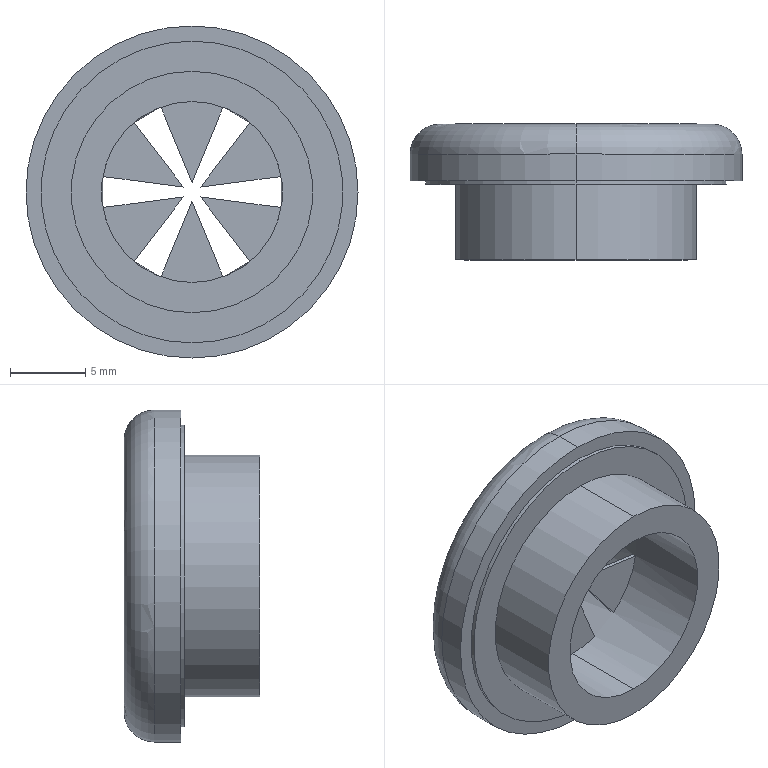Part | SolidWorks | features ICE 4, Extrusion 1, Fillet 1 | 1 solid | 38 faces | box 22 x 9 x 22 mm | volume 1452 mm3 | plane 28 | cylinder 8 | torus 2 | commonest cylinder face diameters 12 x2 16 x2 20 x2 22 x2
STEP:
#1=CARTESIAN_POINT('',(0.,7.,-11.));
#2=VERTEX_POINT('',#1);
#3=CARTESIAN_POINT('',(0.,7.,11.));
#4=VERTEX_POINT('',#3);
#5=CARTESIAN_POINT('',(0.,7.,0.));
#6=DIRECTION('',(0.,-1.,0.));
#7=DIRECTION('',(0.,0.,1.));
#8=AXIS2_PLACEMENT_3D('',#5,#6,#7);
#9=CIRCLE('',#8,11.);
#10=EDGE_CURVE('',#2,#4,#9,.T.);
#11=ORIENTED_EDGE('',*,*,#10,.F.);
#12=CARTESIAN_POINT('',(0.,9.,-9.));
#13=VERTEX_POINT('',#12);
#14=CARTESIAN_POINT('',(0.,7.,-9.));
#15=DIRECTION('',(1.,0.,0.));
#16=DIRECTION('',(0.,0.,-1.));
#17=AXIS2_PLACEMENT_3D('',#14,#15,#16);
#18=CIRCLE('',#17,2.);
#19=EDGE_CURVE('',#2,#13,#18,.T.);
#20=ORIENTED_EDGE('',*,*,#19,.T.);
#21=CARTESIAN_POINT('',(0.,9.,9.));
#22=VERTEX_POINT('',#21);
#23=CARTESIAN_POINT('',(0.,9.,0.));
#24=DIRECTION('',(0.,1.,0.));
#25=DIRECTION('',(0.,0.,1.));
#26=AXIS2_PLACEMENT_3D('',#23,#24,#25);
#27=CIRCLE('',#26,9.);
#28=EDGE_CURVE('',#22,#13,#27,.T.);
#29=ORIENTED_EDGE('',*,*,#28,.F.);
#30=CARTESIAN_POINT('',(0.,7.,9.));
#31=DIRECTION('',(-1.,0.,0.));
#32=DIRECTION('',(0.,0.,1.));
#33=AXIS2_PLACEMENT_3D('',#30,#31,#32);
#34=CIRCLE('',#33,2.);
#35=EDGE_CURVE('',#4,#22,#34,.T.);
#36=ORIENTED_EDGE('',*,*,#35,.F.);
#37=EDGE_LOOP('',(#11,#20,#29,#36));
#38=FACE_OUTER_BOUND('',#37,.T.);
#39=CARTESIAN_POINT('',(0.,7.,0.));
#40=DIRECTION('',(0.,1.,0.));
#41=DIRECTION('',(0.,0.,1.));
#42=AXIS2_PLACEMENT_3D('',#39,#40,#41);
#43=TOROIDAL_SURFACE('',#42,9.,2.);
#44=ADVANCED_FACE('',(#38),#43,.T.);
#45=CARTESIAN_POINT('',(0.,5.25,-10.));
#46=VERTEX_POINT('',#45);
#47=CARTESIAN_POINT('',(0.,5.25,10.));
#48=VERTEX_POINT('',#47);
#49=CARTESIAN_POINT('',(0.,5.25,0.));
#50=DIRECTION('',(0.,-1.,0.));
#51=DIRECTION('',(0.,0.,-1.));
#52=AXIS2_PLACEMENT_3D('',#49,#50,#51);
#53=CIRCLE('',#52,10.);
#54=EDGE_CURVE('',#46,#48,#53,.T.);
#55=ORIENTED_EDGE('',*,*,#54,.T.);
#56=CARTESIAN_POINT('',(0.,5.,10.));
#57=VERTEX_POINT('',#56);
#58=CARTESIAN_POINT('',(0.,5.25,10.));
#59=DIRECTION('',(0.,-1.,0.));
#60=VECTOR('',#59,1000.);
#61=LINE('',#58,#60);
#62=EDGE_CURVE('',#48,#57,#61,.T.);
#63=ORIENTED_EDGE('',*,*,#62,.T.);
#64=CARTESIAN_POINT('',(0.,5.,-10.));
#65=VERTEX_POINT('',#64);
#66=CARTESIAN_POINT('',(0.,5.,0.));
#67=DIRECTION('',(0.,-1.,0.));
#68=DIRECTION('',(0.,0.,-1.));
#69=AXIS2_PLACEMENT_3D('',#66,#67,#68);
#70=CIRCLE('',#69,10.);
#71=EDGE_CURVE('',#65,#57,#70,.T.);
#72=ORIENTED_EDGE('',*,*,#71,.F.);
#73=CARTESIAN_POINT('',(0.,5.25,-10.));
#74=DIRECTION('',(0.,-1.,0.));
#75=VECTOR('',#74,1000.);
#76=LINE('',#73,#75);
#77=EDGE_CURVE('',#46,#65,#76,.T.);
#78=ORIENTED_EDGE('',*,*,#77,.F.);
#79=EDGE_LOOP('',(#55,#63,#72,#78));
#80=FACE_OUTER_BOUND('',#79,.T.);
#81=CARTESIAN_POINT('',(0.,5.25,0.));
#82=DIRECTION('',(0.,-1.,0.));
#83=DIRECTION('',(0.,0.,-1.));
#84=AXIS2_PLACEMENT_3D('',#81,#82,#83);
#85=CYLINDRICAL_SURFACE('',#84,10.);
#86=ADVANCED_FACE('',(#80),#85,.T.);
#87=CARTESIAN_POINT('',(0.,5.,8.));
#88=VERTEX_POINT('',#87);
#89=CARTESIAN_POINT('',(0.,5.,-8.));
#90=VERTEX_POINT('',#89);
#91=CARTESIAN_POINT('',(0.,5.,0.));
#92=DIRECTION('',(0.,1.,0.));
#93=DIRECTION('',(0.,0.,1.));
#94=AXIS2_PLACEMENT_3D('',#91,#92,#93);
#95=CIRCLE('',#94,8.);
#96=EDGE_CURVE('',#88,#90,#95,.T.);
#97=ORIENTED_EDGE('',*,*,#96,.F.);
#98=CARTESIAN_POINT('',(0.,0.,8.));
#99=VERTEX_POINT('',#98);
#100=CARTESIAN_POINT('',(0.,5.,8.));
#101=DIRECTION('',(0.,-1.,0.));
#102=VECTOR('',#101,1000.);
#103=LINE('',#100,#102);
#104=EDGE_CURVE('',#88,#99,#103,.T.);
#105=ORIENTED_EDGE('',*,*,#104,.T.);
#106=CARTESIAN_POINT('',(0.,0.,-8.));
#107=VERTEX_POINT('',#106);
#108=CARTESIAN_POINT('',(0.,0.,0.));
#109=DIRECTION('',(0.,1.,0.));
#110=DIRECTION('',(0.,0.,1.));
#111=AXIS2_PLACEMENT_3D('',#108,#109,#110);
#112=CIRCLE('',#111,8.);
#113=EDGE_CURVE('',#99,#107,#112,.T.);
#114=ORIENTED_EDGE('',*,*,#113,.T.);
#115=CARTESIAN_POINT('',(0.,5.,-8.));
#116=DIRECTION('',(0.,-1.,0.));
#117=VECTOR('',#116,1000.);
#118=LINE('',#115,#117);
#119=EDGE_CURVE('',#90,#107,#118,.T.);
#120=ORIENTED_EDGE('',*,*,#119,.F.);
#121=EDGE_LOOP('',(#97,#105,#114,#120));
#122=FACE_OUTER_BOUND('',#121,.T.);
#123=CARTESIAN_POINT('',(0.,5.,0.));
#124=DIRECTION('',(0.,-1.,0.));
#125=DIRECTION('',(0.,0.,-1.));
#126=AXIS2_PLACEMENT_3D('',#123,#124,#125);
#127=CYLINDRICAL_SURFACE('',#126,8.);
#128=ADVANCED_FACE('',(#122),#127,.T.);
#129=CARTESIAN_POINT('',(-3.847,5.75,4.605));
#130=VERTEX_POINT('',#129);
#131=CARTESIAN_POINT('',(-5.911,5.75,1.029));
#132=VERTEX_POINT('',#131);
#133=CARTESIAN_POINT('',(0.,5.75,0.));
#134=DIRECTION('',(0.,-1.,0.));
#135=DIRECTION('',(0.,0.,1.));
#136=AXIS2_PLACEMENT_3D('',#133,#134,#135);
#137=CIRCLE('',#136,6.);
#138=EDGE_CURVE('',#130,#132,#137,.T.);
#139=ORIENTED_EDGE('',*,*,#138,.F.);
#140=CARTESIAN_POINT('',(-3.847,6.,4.605));
#141=VERTEX_POINT('',#140);
#142=CARTESIAN_POINT('',(-3.847,5.75,4.605));
#143=DIRECTION('',(0.,1.,0.));
#144=VECTOR('',#143,1000.);
#145=LINE('',#142,#144);
#146=EDGE_CURVE('',#130,#141,#145,.T.);
#147=ORIENTED_EDGE('',*,*,#146,.T.);
#148=CARTESIAN_POINT('',(-5.911,6.,1.029));
#149=VERTEX_POINT('',#148);
#150=CARTESIAN_POINT('',(0.,6.,0.));
#151=DIRECTION('',(0.,-1.,0.));
#152=DIRECTION('',(0.,0.,1.));
#153=AXIS2_PLACEMENT_3D('',#150,#151,#152);
#154=CIRCLE('',#153,6.);
#155=EDGE_CURVE('',#141,#149,#154,.T.);
#156=ORIENTED_EDGE('',*,*,#155,.T.);
#157=CARTESIAN_POINT('',(-5.911,5.75,1.029));
#158=DIRECTION('',(0.,1.,0.));
#159=VECTOR('',#158,1000.);
#160=LINE('',#157,#159);
#161=EDGE_CURVE('',#132,#149,#160,.T.);
#162=ORIENTED_EDGE('',*,*,#161,.F.);
#163=EDGE_LOOP('',(#139,#147,#156,#162));
#164=FACE_BOUND('',#163,.T.);
#165=CARTESIAN_POINT('',(-5.911,5.75,-1.029));
#166=VERTEX_POINT('',#165);
#167=CARTESIAN_POINT('',(-3.847,5.75,-4.605));
#168=VERTEX_POINT('',#167);
#169=CARTESIAN_POINT('',(0.,5.75,0.));
#170=DIRECTION('',(0.,-1.,0.));
#171=DIRECTION('',(0.,0.,1.));
#172=AXIS2_PLACEMENT_3D('',#169,#170,#171);
#173=CIRCLE('',#172,6.);
#174=EDGE_CURVE('',#166,#168,#173,.T.);
#175=ORIENTED_EDGE('',*,*,#174,.F.);
#176=CARTESIAN_POINT('',(-5.911,6.,-1.029));
#177=VERTEX_POINT('',#176);
#178=CARTESIAN_POINT('',(-5.911,5.75,-1.029));
#179=DIRECTION('',(0.,1.,0.));
#180=VECTOR('',#179,1000.);
#181=LINE('',#178,#180);
#182=EDGE_CURVE('',#166,#177,#181,.T.);
#183=ORIENTED_EDGE('',*,*,#182,.T.);
#184=CARTESIAN_POINT('',(-3.847,6.,-4.605));
#185=VERTEX_POINT('',#184);
#186=CARTESIAN_POINT('',(0.,6.,0.));
#187=DIRECTION('',(0.,-1.,0.));
#188=DIRECTION('',(0.,0.,1.));
#189=AXIS2_PLACEMENT_3D('',#186,#187,#188);
#190=CIRCLE('',#189,6.);
#191=EDGE_CURVE('',#177,#185,#190,.T.);
#192=ORIENTED_EDGE('',*,*,#191,.T.);
#193=CARTESIAN_POINT('',(-3.847,5.75,-4.605));
#194=DIRECTION('',(0.,1.,0.));
#195=VECTOR('',#194,1000.);
#196=LINE('',#193,#195);
#197=EDGE_CURVE('',#168,#185,#196,.T.);
#198=ORIENTED_EDGE('',*,*,#197,.F.);
#199=EDGE_LOOP('',(#175,#183,#192,#198));
#200=FACE_BOUND('',#199,.T.);
#201=CARTESIAN_POINT('',(0.,0.,6.));
#202=VERTEX_POINT('',#201);
#203=CARTESIAN_POINT('',(0.,0.,-6.));
#204=VERTEX_POINT('',#203);
#205=CARTESIAN_POINT('',(0.,0.,0.));
#206=DIRECTION('',(0.,-1.,0.));
#207=DIRECTION('',(0.,0.,1.));
#208=AXIS2_PLACEMENT_3D('',#205,#206,#207);
#209=CIRCLE('',#208,6.);
#210=EDGE_CURVE('',#202,#204,#209,.T.);
#211=ORIENTED_EDGE('',*,*,#210,.T.);
#212=CARTESIAN_POINT('',(0.,5.75,-6.));
#213=VERTEX_POINT('',#212);
#214=CARTESIAN_POINT('',(0.,-0.001,-6.));
#215=DIRECTION('',(0.,1.,0.));
#216=VECTOR('',#215,1000.);
#217=LINE('',#214,#216);
#218=EDGE_CURVE('',#204,#213,#217,.T.);
#219=ORIENTED_EDGE('',*,*,#218,.T.);
#220=CARTESIAN_POINT('',(-2.064,5.75,-5.634));
#221=VERTEX_POINT('',#220);
#222=CARTESIAN_POINT('',(0.,5.75,0.));
#223=DIRECTION('',(0.,-1.,0.));
#224=DIRECTION('',(0.,0.,1.));
#225=AXIS2_PLACEMENT_3D('',#222,#223,#224);
#226=CIRCLE('',#225,6.);
#227=EDGE_CURVE('',#221,#213,#226,.T.);
#228=ORIENTED_EDGE('',*,*,#227,.F.);
#229=CARTESIAN_POINT('',(-2.064,6.,-5.634));
#230=VERTEX_POINT('',#229);
#231=CARTESIAN_POINT('',(-2.064,5.75,-5.634));
#232=DIRECTION('',(0.,1.,0.));
#233=VECTOR('',#232,1000.);
#234=LINE('',#231,#233);
#235=EDGE_CURVE('',#221,#230,#234,.T.);
#236=ORIENTED_EDGE('',*,*,#235,.T.);
#237=CARTESIAN_POINT('',(0.,6.,-6.));
#238=VERTEX_POINT('',#237);
#239=CARTESIAN_POINT('',(0.,6.,0.));
#240=DIRECTION('',(0.,-1.,0.));
#241=DIRECTION('',(0.,0.,1.));
#242=AXIS2_PLACEMENT_3D('',#239,#240,#241);
#243=CIRCLE('',#242,6.);
#244=EDGE_CURVE('',#230,#238,#243,.T.);
#245=ORIENTED_EDGE('',*,*,#244,.T.);
#246=CARTESIAN_POINT('',(0.,9.,-6.));
#247=VERTEX_POINT('',#246);
#248=CARTESIAN_POINT('',(0.,-0.001,-6.));
#249=DIRECTION('',(0.,1.,0.));
#250=VECTOR('',#249,1000.);
#251=LINE('',#248,#250);
#252=EDGE_CURVE('',#238,#247,#251,.T.);
#253=ORIENTED_EDGE('',*,*,#252,.T.);
#254=CARTESIAN_POINT('',(0.,9.,6.));
#255=VERTEX_POINT('',#254);
#256=CARTESIAN_POINT('',(0.,9.,0.));
#257=DIRECTION('',(0.,1.,0.));
#258=DIRECTION('',(0.,0.,1.));
#259=AXIS2_PLACEMENT_3D('',#256,#257,#258);
#260=CIRCLE('',#259,6.);
#261=EDGE_CURVE('',#247,#255,#260,.T.);
#262=ORIENTED_EDGE('',*,*,#261,.T.);
#263=CARTESIAN_POINT('',(0.,6.,6.));
#264=VERTEX_POINT('',#263);
#265=CARTESIAN_POINT('',(0.,-0.001,6.));
#266=DIRECTION('',(0.,1.,0.));
#267=VECTOR('',#266,1000.);
#268=LINE('',#265,#267);
#269=EDGE_CURVE('',#264,#255,#268,.T.);
#270=ORIENTED_EDGE('',*,*,#269,.F.);
#271=CARTESIAN_POINT('',(-2.064,6.,5.634));
#272=VERTEX_POINT('',#271);
#273=CARTESIAN_POINT('',(0.,6.,0.));
#274=DIRECTION('',(0.,-1.,0.));
#275=DIRECTION('',(0.,0.,1.));
#276=AXIS2_PLACEMENT_3D('',#273,#274,#275);
#277=CIRCLE('',#276,6.);
#278=EDGE_CURVE('',#264,#272,#277,.T.);
#279=ORIENTED_EDGE('',*,*,#278,.T.);
#280=CARTESIAN_POINT('',(-2.064,5.75,5.634));
#281=VERTEX_POINT('',#280);
#282=CARTESIAN_POINT('',(-2.064,5.75,5.634));
#283=DIRECTION('',(0.,1.,0.));
#284=VECTOR('',#283,1000.);
#285=LINE('',#282,#284);
#286=EDGE_CURVE('',#281,#272,#285,.T.);
#287=ORIENTED_EDGE('',*,*,#286,.F.);
#288=CARTESIAN_POINT('',(0.,5.75,6.));
#289=VERTEX_POINT('',#288);
#290=CARTESIAN_POINT('',(0.,5.75,0.));
#291=DIRECTION('',(0.,-1.,0.));
#292=DIRECTION('',(0.,0.,1.));
#293=AXIS2_PLACEMENT_3D('',#290,#291,#292);
#294=CIRCLE('',#293,6.);
#295=EDGE_CURVE('',#289,#281,#294,.T.);
#296=ORIENTED_EDGE('',*,*,#295,.F.);
#297=CARTESIAN_POINT('',(0.,-0.001,6.));
#298=DIRECTION('',(0.,1.,0.));
#299=VECTOR('',#298,1000.);
#300=LINE('',#297,#299);
#301=EDGE_CURVE('',#202,#289,#300,.T.);
#302=ORIENTED_EDGE('',*,*,#301,.F.);
#303=EDGE_LOOP('',(#211,#219,#228,#236,#245,#253,#262,#270,#279,#287,#296,#302));
#304=FACE_OUTER_BOUND('',#303,.T.);
#305=CARTESIAN_POINT('',(0.,-0.001,0.));
#306=DIRECTION('',(0.,1.,0.));
#307=DIRECTION('',(0.,0.,1.));
#308=AXIS2_PLACEMENT_3D('',#305,#306,#307);
#309=CYLINDRICAL_SURFACE('',#308,6.);
#310=ADVANCED_FACE('',(#164,#200,#304),#309,.F.);
#311=ORIENTED_EDGE('',*,*,#10,.T.);
#312=CARTESIAN_POINT('',(0.,5.25,11.));
#313=VERTEX_POINT('',#312);
#314=CARTESIAN_POINT('',(0.,9.,11.));
#315=DIRECTION('',(0.,-1.,0.));
#316=VECTOR('',#315,1000.);
#317=LINE('',#314,#316);
#318=EDGE_CURVE('',#4,#313,#317,.T.);
#319=ORIENTED_EDGE('',*,*,#318,.T.);
#320=CARTESIAN_POINT('',(0.,5.25,-11.));
#321=VERTEX_POINT('',#320);
#322=CARTESIAN_POINT('',(0.,5.25,0.));
#323=DIRECTION('',(0.,-1.,0.));
#324=DIRECTION('',(0.,0.,-1.));
#325=AXIS2_PLACEMENT_3D('',#322,#323,#324);
#326=CIRCLE('',#325,11.);
#327=EDGE_CURVE('',#321,#313,#326,.T.);
#328=ORIENTED_EDGE('',*,*,#327,.F.);
#329=CARTESIAN_POINT('',(0.,9.,-11.));
#330=DIRECTION('',(0.,-1.,0.));
#331=VECTOR('',#330,1000.);
#332=LINE('',#329,#331);
#333=EDGE_CURVE('',#2,#321,#332,.T.);
#334=ORIENTED_EDGE('',*,*,#333,.F.);
#335=EDGE_LOOP('',(#311,#319,#328,#334));
#336=FACE_OUTER_BOUND('',#335,.T.);
#337=CARTESIAN_POINT('',(0.,9.,0.));
#338=DIRECTION('',(0.,-1.,0.));
#339=DIRECTION('',(0.,0.,-1.));
#340=AXIS2_PLACEMENT_3D('',#337,#338,#339);
#341=CYLINDRICAL_SURFACE('',#340,11.);
#342=ADVANCED_FACE('',(#336),#341,.T.);
#343=ORIENTED_EDGE('',*,*,#318,.F.);
#344=CARTESIAN_POINT('',(0.,7.,0.));
#345=DIRECTION('',(0.,-1.,0.));
#346=DIRECTION('',(0.,0.,1.));
#347=AXIS2_PLACEMENT_3D('',#344,#345,#346);
#348=CIRCLE('',#347,11.);
#349=EDGE_CURVE('',#4,#2,#348,.T.);
#350=ORIENTED_EDGE('',*,*,#349,.T.);
#351=ORIENTED_EDGE('',*,*,#333,.T.);
#352=CARTESIAN_POINT('',(0.,5.25,0.));
#353=DIRECTION('',(0.,-1.,0.));
#354=DIRECTION('',(0.,0.,-1.));
#355=AXIS2_PLACEMENT_3D('',#352,#353,#354);
#356=CIRCLE('',#355,11.);
#357=EDGE_CURVE('',#313,#321,#356,.T.);
#358=ORIENTED_EDGE('',*,*,#357,.F.);
#359=EDGE_LOOP('',(#343,#350,#351,#358));
#360=FACE_OUTER_BOUND('',#359,.T.);
#361=CARTESIAN_POINT('',(0.,9.,0.));
#362=DIRECTION('',(0.,-1.,0.));
#363=DIRECTION('',(0.,0.,-1.));
#364=AXIS2_PLACEMENT_3D('',#361,#362,#363);
#365=CYLINDRICAL_SURFACE('',#364,11.);
#366=ADVANCED_FACE('',(#360),#365,.T.);
#367=CARTESIAN_POINT('',(0.,5.,0.));
#368=DIRECTION('',(0.,1.,0.));
#369=DIRECTION('',(0.,0.,1.));
#370=AXIS2_PLACEMENT_3D('',#367,#368,#369);
#371=CIRCLE('',#370,8.);
#372=EDGE_CURVE('',#90,#88,#371,.T.);
#373=ORIENTED_EDGE('',*,*,#372,.T.);
#374=ORIENTED_EDGE('',*,*,#96,.T.);
#375=EDGE_LOOP('',(#373,#374));
#376=FACE_BOUND('',#375,.T.);
#377=ORIENTED_EDGE('',*,*,#71,.T.);
#378=CARTESIAN_POINT('',(0.,5.,0.));
#379=DIRECTION('',(0.,-1.,0.));
#380=DIRECTION('',(0.,0.,-1.));
#381=AXIS2_PLACEMENT_3D('',#378,#379,#380);
#382=CIRCLE('',#381,10.);
#383=EDGE_CURVE('',#57,#65,#382,.T.);
#384=ORIENTED_EDGE('',*,*,#383,.T.);
#385=EDGE_LOOP('',(#377,#384));
#386=FACE_OUTER_BOUND('',#385,.T.);
#387=CARTESIAN_POINT('',(0.,5.,0.));
#388=DIRECTION('',(0.,1.,0.));
#389=DIRECTION('',(0.,0.,1.));
#390=AXIS2_PLACEMENT_3D('',#387,#388,#389);
#391=PLANE('',#390);
#392=ADVANCED_FACE('',(#376,#386),#391,.F.);
#393=ORIENTED_EDGE('',*,*,#218,.F.);
#394=CARTESIAN_POINT('',(0.,0.,0.));
#395=DIRECTION('',(0.,-1.,0.));
#396=DIRECTION('',(0.,0.,1.));
#397=AXIS2_PLACEMENT_3D('',#394,#395,#396);
#398=CIRCLE('',#397,6.);
#399=EDGE_CURVE('',#204,#202,#398,.T.);
#400=ORIENTED_EDGE('',*,*,#399,.T.);
#401=ORIENTED_EDGE('',*,*,#301,.T.);
#402=CARTESIAN_POINT('',(2.064,5.75,5.634));
#403=VERTEX_POINT('',#402);
#404=CARTESIAN_POINT('',(0.,5.75,0.));
#405=DIRECTION('',(0.,-1.,0.));
#406=DIRECTION('',(0.,0.,1.));
#407=AXIS2_PLACEMENT_3D('',#404,#405,#406);
#408=CIRCLE('',#407,6.);
#409=EDGE_CURVE('',#403,#289,#408,.T.);
#410=ORIENTED_EDGE('',*,*,#409,.F.);
#411=CARTESIAN_POINT('',(2.064,6.,5.634));
#412=VERTEX_POINT('',#411);
#413=CARTESIAN_POINT('',(2.064,5.75,5.634));
#414=DIRECTION('',(0.,1.,0.));
#415=VECTOR('',#414,1000.);
#416=LINE('',#413,#415);
#417=EDGE_CURVE('',#403,#412,#416,.T.);
#418=ORIENTED_EDGE('',*,*,#417,.T.);
#419=CARTESIAN_POINT('',(0.,6.,0.));
#420=DIRECTION('',(0.,-1.,0.));
#421=DIRECTION('',(0.,0.,1.));
#422=AXIS2_PLACEMENT_3D('',#419,#420,#421);
#423=CIRCLE('',#422,6.);
#424=EDGE_CURVE('',#412,#264,#423,.T.);
#425=ORIENTED_EDGE('',*,*,#424,.T.);
#426=ORIENTED_EDGE('',*,*,#269,.T.);
#427=CARTESIAN_POINT('',(0.,9.,0.));
#428=DIRECTION('',(0.,1.,0.));
#429=DIRECTION('',(0.,0.,1.));
#430=AXIS2_PLACEMENT_3D('',#427,#428,#429);
#431=CIRCLE('',#430,6.);
#432=EDGE_CURVE('',#255,#247,#431,.T.);
#433=ORIENTED_EDGE('',*,*,#432,.T.);
#434=ORIENTED_EDGE('',*,*,#252,.F.);
#435=CARTESIAN_POINT('',(2.064,6.,-5.634));
#436=VERTEX_POINT('',#435);
#437=CARTESIAN_POINT('',(0.,6.,0.));
#438=DIRECTION('',(0.,-1.,0.));
#439=DIRECTION('',(0.,0.,1.));
#440=AXIS2_PLACEMENT_3D('',#437,#438,#439);
#441=CIRCLE('',#440,6.);
#442=EDGE_CURVE('',#238,#436,#441,.T.);
#443=ORIENTED_EDGE('',*,*,#442,.T.);
#444=CARTESIAN_POINT('',(2.064,5.75,-5.634));
#445=VERTEX_POINT('',#444);
#446=CARTESIAN_POINT('',(2.064,5.75,-5.634));
#447=DIRECTION('',(0.,1.,0.));
#448=VECTOR('',#447,1000.);
#449=LINE('',#446,#448);
#450=EDGE_CURVE('',#445,#436,#449,.T.);
#451=ORIENTED_EDGE('',*,*,#450,.F.);
#452=CARTESIAN_POINT('',(0.,5.75,0.));
#453=DIRECTION('',(0.,-1.,0.));
#454=DIRECTION('',(0.,0.,1.));
#455=AXIS2_PLACEMENT_3D('',#452,#453,#454);
#456=CIRCLE('',#455,6.);
#457=EDGE_CURVE('',#213,#445,#456,.T.);
#458=ORIENTED_EDGE('',*,*,#457,.F.);
#459=EDGE_LOOP('',(#393,#400,#401,#410,#418,#425,#426,#433,#434,#443,#451,#458));
#460=FACE_OUTER_BOUND('',#459,.T.);
#461=CARTESIAN_POINT('',(3.847,5.75,-4.605));
#462=VERTEX_POINT('',#461);
#463=CARTESIAN_POINT('',(5.911,5.75,-1.029));
#464=VERTEX_POINT('',#463);
#465=CARTESIAN_POINT('',(0.,5.75,0.));
#466=DIRECTION('',(0.,-1.,0.));
#467=DIRECTION('',(0.,0.,1.));
#468=AXIS2_PLACEMENT_3D('',#465,#466,#467);
#469=CIRCLE('',#468,6.);
#470=EDGE_CURVE('',#462,#464,#469,.T.);
#471=ORIENTED_EDGE('',*,*,#470,.F.);
#472=CARTESIAN_POINT('',(3.847,6.,-4.605));
#473=VERTEX_POINT('',#472);
#474=CARTESIAN_POINT('',(3.847,5.75,-4.605));
#475=DIRECTION('',(0.,1.,0.));
#476=VECTOR('',#475,1000.);
#477=LINE('',#474,#476);
#478=EDGE_CURVE('',#462,#473,#477,.T.);
#479=ORIENTED_EDGE('',*,*,#478,.T.);
#480=CARTESIAN_POINT('',(5.911,6.,-1.029));
#481=VERTEX_POINT('',#480);
#482=CARTESIAN_POINT('',(0.,6.,0.));
#483=DIRECTION('',(0.,-1.,0.));
#484=DIRECTION('',(0.,0.,1.));
#485=AXIS2_PLACEMENT_3D('',#482,#483,#484);
#486=CIRCLE('',#485,6.);
#487=EDGE_CURVE('',#473,#481,#486,.T.);
#488=ORIENTED_EDGE('',*,*,#487,.T.);
#489=CARTESIAN_POINT('',(5.911,5.75,-1.029));
#490=DIRECTION('',(0.,1.,0.));
#491=VECTOR('',#490,1000.);
#492=LINE('',#489,#491);
#493=EDGE_CURVE('',#464,#481,#492,.T.);
#494=ORIENTED_EDGE('',*,*,#493,.F.);
#495=EDGE_LOOP('',(#471,#479,#488,#494));
#496=FACE_BOUND('',#495,.T.);
#497=CARTESIAN_POINT('',(5.911,5.75,1.029));
#498=VERTEX_POINT('',#497);
#499=CARTESIAN_POINT('',(3.847,5.75,4.605));
#500=VERTEX_POINT('',#499);
#501=CARTESIAN_POINT('',(0.,5.75,0.));
#502=DIRECTION('',(0.,-1.,0.));
#503=DIRECTION('',(0.,0.,1.));
#504=AXIS2_PLACEMENT_3D('',#501,#502,#503);
#505=CIRCLE('',#504,6.);
#506=EDGE_CURVE('',#498,#500,#505,.T.);
#507=ORIENTED_EDGE('',*,*,#506,.F.);
#508=CARTESIAN_POINT('',(5.911,6.,1.029));
#509=VERTEX_POINT('',#508);
#510=CARTESIAN_POINT('',(5.911,5.75,1.029));
#511=DIRECTION('',(0.,1.,0.));
#512=VECTOR('',#511,1000.);
#513=LINE('',#510,#512);
#514=EDGE_CURVE('',#498,#509,#513,.T.);
#515=ORIENTED_EDGE('',*,*,#514,.T.);
#516=CARTESIAN_POINT('',(3.847,6.,4.605));
#517=VERTEX_POINT('',#516);
#518=CARTESIAN_POINT('',(0.,6.,0.));
#519=DIRECTION('',(0.,-1.,0.));
#520=DIRECTION('',(0.,0.,1.));
#521=AXIS2_PLACEMENT_3D('',#518,#519,#520);
#522=CIRCLE('',#521,6.);
#523=EDGE_CURVE('',#509,#517,#522,.T.);
#524=ORIENTED_EDGE('',*,*,#523,.T.);
#525=CARTESIAN_POINT('',(3.847,5.75,4.605));
#526=DIRECTION('',(0.,1.,0.));
#527=VECTOR('',#526,1000.);
#528=LINE('',#525,#527);
#529=EDGE_CURVE('',#500,#517,#528,.T.);
#530=ORIENTED_EDGE('',*,*,#529,.F.);
#531=EDGE_LOOP('',(#507,#515,#524,#530));
#532=FACE_BOUND('',#531,.T.);
#533=CARTESIAN_POINT('',(0.,-0.001,0.));
#534=DIRECTION('',(0.,1.,0.));
#535=DIRECTION('',(0.,0.,1.));
#536=AXIS2_PLACEMENT_3D('',#533,#534,#535);
#537=CYLINDRICAL_SURFACE('',#536,6.);
#538=ADVANCED_FACE('',(#460,#496,#532),#537,.F.);
#539=ORIENTED_EDGE('',*,*,#104,.F.);
#540=ORIENTED_EDGE('',*,*,#372,.F.);
#541=ORIENTED_EDGE('',*,*,#119,.T.);
#542=CARTESIAN_POINT('',(0.,0.,0.));
#543=DIRECTION('',(0.,1.,0.));
#544=DIRECTION('',(0.,0.,1.));
#545=AXIS2_PLACEMENT_3D('',#542,#543,#544);
#546=CIRCLE('',#545,8.);
#547=EDGE_CURVE('',#107,#99,#546,.T.);
#548=ORIENTED_EDGE('',*,*,#547,.T.);
#549=EDGE_LOOP('',(#539,#540,#541,#548));
#550=FACE_OUTER_BOUND('',#549,.T.);
#551=CARTESIAN_POINT('',(0.,5.,0.));
#552=DIRECTION('',(0.,-1.,0.));
#553=DIRECTION('',(0.,0.,-1.));
#554=AXIS2_PLACEMENT_3D('',#551,#552,#553);
#555=CYLINDRICAL_SURFACE('',#554,8.);
#556=ADVANCED_FACE('',(#550),#555,.T.);
#557=ORIENTED_EDGE('',*,*,#210,.F.);
#558=ORIENTED_EDGE('',*,*,#399,.F.);
#559=EDGE_LOOP('',(#557,#558));
#560=FACE_BOUND('',#559,.T.);
#561=ORIENTED_EDGE('',*,*,#547,.F.);
#562=ORIENTED_EDGE('',*,*,#113,.F.);
#563=EDGE_LOOP('',(#561,#562));
#564=FACE_OUTER_BOUND('',#563,.T.);
#565=CARTESIAN_POINT('',(0.,0.,0.));
#566=DIRECTION('',(0.,1.,0.));
#567=DIRECTION('',(0.,0.,1.));
#568=AXIS2_PLACEMENT_3D('',#565,#566,#567);
#569=PLANE('',#568);
#570=ADVANCED_FACE('',(#560,#564),#569,.F.);
#571=ORIENTED_EDGE('',*,*,#28,.T.);
#572=CARTESIAN_POINT('',(0.,9.,0.));
#573=DIRECTION('',(0.,1.,0.));
#574=DIRECTION('',(0.,0.,1.));
#575=AXIS2_PLACEMENT_3D('',#572,#573,#574);
#576=CIRCLE('',#575,9.);
#577=EDGE_CURVE('',#13,#22,#576,.T.);
#578=ORIENTED_EDGE('',*,*,#577,.T.);
#579=EDGE_LOOP('',(#571,#578));
#580=FACE_OUTER_BOUND('',#579,.T.);
#581=ORIENTED_EDGE('',*,*,#432,.F.);
#582=ORIENTED_EDGE('',*,*,#261,.F.);
#583=EDGE_LOOP('',(#581,#582));
#584=FACE_BOUND('',#583,.T.);
#585=CARTESIAN_POINT('',(0.,9.,0.));
#586=DIRECTION('',(0.,1.,0.));
#587=DIRECTION('',(0.,0.,1.));
#588=AXIS2_PLACEMENT_3D('',#585,#586,#587);
#589=PLANE('',#588);
#590=ADVANCED_FACE('',(#580,#584),#589,.T.);
#591=CARTESIAN_POINT('',(0.,6.,0.65));
#592=VERTEX_POINT('',#591);
#593=CARTESIAN_POINT('',(0.,6.,0.65));
#594=DIRECTION('',(0.3827,0.,0.9239));
#595=VECTOR('',#594,1000.);
#596=LINE('',#593,#595);
#597=EDGE_CURVE('',#592,#412,#596,.T.);
#598=ORIENTED_EDGE('',*,*,#597,.T.);
#599=ORIENTED_EDGE('',*,*,#417,.F.);
#600=CARTESIAN_POINT('',(0.,5.75,0.65));
#601=VERTEX_POINT('',#600);
#602=CARTESIAN_POINT('',(0.,5.75,0.65));
#603=DIRECTION('',(0.3827,0.,0.9239));
#604=VECTOR('',#603,1000.);
#605=LINE('',#602,#604);
#606=EDGE_CURVE('',#601,#403,#605,.T.);
#607=ORIENTED_EDGE('',*,*,#606,.F.);
#608=CARTESIAN_POINT('',(0.,5.75,0.65));
#609=DIRECTION('',(0.,1.,0.));
#610=VECTOR('',#609,1000.);
#611=LINE('',#608,#610);
#612=EDGE_CURVE('',#601,#592,#611,.T.);
#613=ORIENTED_EDGE('',*,*,#612,.T.);
#614=EDGE_LOOP('',(#598,#599,#607,#613));
#615=FACE_OUTER_BOUND('',#614,.T.);
#616=CARTESIAN_POINT('',(0.,5.75,0.65));
#617=DIRECTION('',(-0.9239,0.,0.3827));
#618=DIRECTION('',(0.3827,0.,0.9239));
#619=AXIS2_PLACEMENT_3D('',#616,#617,#618);
#620=PLANE('',#619);
#621=ADVANCED_FACE('',(#615),#620,.F.);
#622=CARTESIAN_POINT('',(0.,6.,0.65));
#623=DIRECTION('',(0.3827,0.,-0.9239));
#624=VECTOR('',#623,1000.);
#625=LINE('',#622,#624);
#626=EDGE_CURVE('',#272,#592,#625,.T.);
#627=ORIENTED_EDGE('',*,*,#626,.T.);
#628=ORIENTED_EDGE('',*,*,#612,.F.);
#629=CARTESIAN_POINT('',(0.,5.75,0.65));
#630=DIRECTION('',(0.3827,0.,-0.9239));
#631=VECTOR('',#630,1000.);
#632=LINE('',#629,#631);
#633=EDGE_CURVE('',#281,#601,#632,.T.);
#634=ORIENTED_EDGE('',*,*,#633,.F.);
#635=ORIENTED_EDGE('',*,*,#286,.T.);
#636=EDGE_LOOP('',(#627,#628,#634,#635));
#637=FACE_OUTER_BOUND('',#636,.T.);
#638=CARTESIAN_POINT('',(0.,5.75,0.65));
#639=DIRECTION('',(0.9239,0.,0.3827));
#640=DIRECTION('',(0.3827,0.,-0.9239));
#641=AXIS2_PLACEMENT_3D('',#638,#639,#640);
#642=PLANE('',#641);
#643=ADVANCED_FACE('',(#637),#642,.F.);
#644=ORIENTED_EDGE('',*,*,#606,.T.);
#645=ORIENTED_EDGE('',*,*,#409,.T.);
#646=ORIENTED_EDGE('',*,*,#295,.T.);
#647=ORIENTED_EDGE('',*,*,#633,.T.);
#648=EDGE_LOOP('',(#644,#645,#646,#647));
#649=FACE_OUTER_BOUND('',#648,.T.);
#650=CARTESIAN_POINT('',(0.,5.75,0.));
#651=DIRECTION('',(0.,1.,0.));
#652=DIRECTION('',(0.,0.,1.));
#653=AXIS2_PLACEMENT_3D('',#650,#651,#652);
#654=PLANE('',#653);
#655=ADVANCED_FACE('',(#649),#654,.F.);
#656=ORIENTED_EDGE('',*,*,#597,.F.);
#657=ORIENTED_EDGE('',*,*,#626,.F.);
#658=ORIENTED_EDGE('',*,*,#278,.F.);
#659=ORIENTED_EDGE('',*,*,#424,.F.);
#660=EDGE_LOOP('',(#656,#657,#658,#659));
#661=FACE_OUTER_BOUND('',#660,.T.);
#662=CARTESIAN_POINT('',(0.,6.,0.));
#663=DIRECTION('',(0.,1.,0.));
#664=DIRECTION('',(0.,0.,1.));
#665=AXIS2_PLACEMENT_3D('',#662,#663,#664);
#666=PLANE('',#665);
#667=ADVANCED_FACE('',(#661),#666,.T.);
#668=CARTESIAN_POINT('',(0.5629,6.,0.325));
#669=VERTEX_POINT('',#668);
#670=CARTESIAN_POINT('',(0.5629,6.,0.325));
#671=DIRECTION('',(0.9914,0.,0.1305));
#672=VECTOR('',#671,1000.);
#673=LINE('',#670,#672);
#674=EDGE_CURVE('',#669,#509,#673,.T.);
#675=ORIENTED_EDGE('',*,*,#674,.T.);
#676=ORIENTED_EDGE('',*,*,#514,.F.);
#677=CARTESIAN_POINT('',(0.5629,5.75,0.325));
#678=VERTEX_POINT('',#677);
#679=CARTESIAN_POINT('',(0.5629,5.75,0.325));
#680=DIRECTION('',(0.9914,0.,0.1305));
#681=VECTOR('',#680,1000.);
#682=LINE('',#679,#681);
#683=EDGE_CURVE('',#678,#498,#682,.T.);
#684=ORIENTED_EDGE('',*,*,#683,.F.);
#685=CARTESIAN_POINT('',(0.5629,5.75,0.325));
#686=DIRECTION('',(0.,1.,0.));
#687=VECTOR('',#686,1000.);
#688=LINE('',#685,#687);
#689=EDGE_CURVE('',#678,#669,#688,.T.);
#690=ORIENTED_EDGE('',*,*,#689,.T.);
#691=EDGE_LOOP('',(#675,#676,#684,#690));
#692=FACE_OUTER_BOUND('',#691,.T.);
#693=CARTESIAN_POINT('',(0.5629,5.75,0.325));
#694=DIRECTION('',(-0.1305,0.,0.9914));
#695=DIRECTION('',(0.9914,0.,0.1305));
#696=AXIS2_PLACEMENT_3D('',#693,#694,#695);
#697=PLANE('',#696);
#698=ADVANCED_FACE('',(#692),#697,.F.);
#699=CARTESIAN_POINT('',(0.5629,6.,0.325));
#700=DIRECTION('',(-0.6088,0.,-0.7934));
#701=VECTOR('',#700,1000.);
#702=LINE('',#699,#701);
#703=EDGE_CURVE('',#517,#669,#702,.T.);
#704=ORIENTED_EDGE('',*,*,#703,.T.);
#705=ORIENTED_EDGE('',*,*,#689,.F.);
#706=CARTESIAN_POINT('',(0.5629,5.75,0.325));
#707=DIRECTION('',(-0.6088,0.,-0.7934));
#708=VECTOR('',#707,1000.);
#709=LINE('',#706,#708);
#710=EDGE_CURVE('',#500,#678,#709,.T.);
#711=ORIENTED_EDGE('',*,*,#710,.F.);
#712=ORIENTED_EDGE('',*,*,#529,.T.);
#713=EDGE_LOOP('',(#704,#705,#711,#712));
#714=FACE_OUTER_BOUND('',#713,.T.);
#715=CARTESIAN_POINT('',(0.5629,5.75,0.325));
#716=DIRECTION('',(0.7934,0.,-0.6088));
#717=DIRECTION('',(-0.6088,0.,-0.7934));
#718=AXIS2_PLACEMENT_3D('',#715,#716,#717);
#719=PLANE('',#718);
#720=ADVANCED_FACE('',(#714),#719,.F.);
#721=ORIENTED_EDGE('',*,*,#683,.T.);
#722=ORIENTED_EDGE('',*,*,#506,.T.);
#723=ORIENTED_EDGE('',*,*,#710,.T.);
#724=EDGE_LOOP('',(#721,#722,#723));
#725=FACE_OUTER_BOUND('',#724,.T.);
#726=CARTESIAN_POINT('',(0.,5.75,0.));
#727=DIRECTION('',(0.,1.,0.));
#728=DIRECTION('',(0.,0.,1.));
#729=AXIS2_PLACEMENT_3D('',#726,#727,#728);
#730=PLANE('',#729);
#731=ADVANCED_FACE('',(#725),#730,.F.);
#732=ORIENTED_EDGE('',*,*,#674,.F.);
#733=ORIENTED_EDGE('',*,*,#703,.F.);
#734=ORIENTED_EDGE('',*,*,#523,.F.);
#735=EDGE_LOOP('',(#732,#733,#734));
#736=FACE_OUTER_BOUND('',#735,.T.);
#737=CARTESIAN_POINT('',(0.,6.,0.));
#738=DIRECTION('',(0.,1.,0.));
#739=DIRECTION('',(0.,0.,1.));
#740=AXIS2_PLACEMENT_3D('',#737,#738,#739);
#741=PLANE('',#740);
#742=ADVANCED_FACE('',(#736),#741,.T.);
#743=CARTESIAN_POINT('',(0.5629,6.,-0.325));
#744=VERTEX_POINT('',#743);
#745=CARTESIAN_POINT('',(0.5629,6.,-0.325));
#746=DIRECTION('',(0.6088,0.,-0.7934));
#747=VECTOR('',#746,1000.);
#748=LINE('',#745,#747);
#749=EDGE_CURVE('',#744,#473,#748,.T.);
#750=ORIENTED_EDGE('',*,*,#749,.T.);
#751=ORIENTED_EDGE('',*,*,#478,.F.);
#752=CARTESIAN_POINT('',(0.5629,5.75,-0.325));
#753=VERTEX_POINT('',#752);
#754=CARTESIAN_POINT('',(0.5629,5.75,-0.325));
#755=DIRECTION('',(0.6088,0.,-0.7934));
#756=VECTOR('',#755,1000.);
#757=LINE('',#754,#756);
#758=EDGE_CURVE('',#753,#462,#757,.T.);
#759=ORIENTED_EDGE('',*,*,#758,.F.);
#760=CARTESIAN_POINT('',(0.5629,5.75,-0.325));
#761=DIRECTION('',(0.,1.,0.));
#762=VECTOR('',#761,1000.);
#763=LINE('',#760,#762);
#764=EDGE_CURVE('',#753,#744,#763,.T.);
#765=ORIENTED_EDGE('',*,*,#764,.T.);
#766=EDGE_LOOP('',(#750,#751,#759,#765));
#767=FACE_OUTER_BOUND('',#766,.T.);
#768=CARTESIAN_POINT('',(0.5629,5.75,-0.325));
#769=DIRECTION('',(0.7934,0.,0.6088));
#770=DIRECTION('',(0.6088,0.,-0.7934));
#771=AXIS2_PLACEMENT_3D('',#768,#769,#770);
#772=PLANE('',#771);
#773=ADVANCED_FACE('',(#767),#772,.F.);
#774=CARTESIAN_POINT('',(0.5629,6.,-0.325));
#775=DIRECTION('',(-0.9914,0.,0.1305));
#776=VECTOR('',#775,1000.);
#777=LINE('',#774,#776);
#778=EDGE_CURVE('',#481,#744,#777,.T.);
#779=ORIENTED_EDGE('',*,*,#778,.T.);
#780=ORIENTED_EDGE('',*,*,#764,.F.);
#781=CARTESIAN_POINT('',(0.5629,5.75,-0.325));
#782=DIRECTION('',(-0.9914,0.,0.1305));
#783=VECTOR('',#782,1000.);
#784=LINE('',#781,#783);
#785=EDGE_CURVE('',#464,#753,#784,.T.);
#786=ORIENTED_EDGE('',*,*,#785,.F.);
#787=ORIENTED_EDGE('',*,*,#493,.T.);
#788=EDGE_LOOP('',(#779,#780,#786,#787));
#789=FACE_OUTER_BOUND('',#788,.T.);
#790=CARTESIAN_POINT('',(0.5629,5.75,-0.325));
#791=DIRECTION('',(-0.1305,0.,-0.9914));
#792=DIRECTION('',(-0.9914,0.,0.1305));
#793=AXIS2_PLACEMENT_3D('',#790,#791,#792);
#794=PLANE('',#793);
#795=ADVANCED_FACE('',(#789),#794,.F.);
#796=ORIENTED_EDGE('',*,*,#758,.T.);
#797=ORIENTED_EDGE('',*,*,#470,.T.);
#798=ORIENTED_EDGE('',*,*,#785,.T.);
#799=EDGE_LOOP('',(#796,#797,#798));
#800=FACE_OUTER_BOUND('',#799,.T.);
#801=CARTESIAN_POINT('',(0.,5.75,0.));
#802=DIRECTION('',(0.,1.,0.));
#803=DIRECTION('',(0.,0.,1.));
#804=AXIS2_PLACEMENT_3D('',#801,#802,#803);
#805=PLANE('',#804);
#806=ADVANCED_FACE('',(#800),#805,.F.);
#807=ORIENTED_EDGE('',*,*,#749,.F.);
#808=ORIENTED_EDGE('',*,*,#778,.F.);
#809=ORIENTED_EDGE('',*,*,#487,.F.);
#810=EDGE_LOOP('',(#807,#808,#809));
#811=FACE_OUTER_BOUND('',#810,.T.);
#812=CARTESIAN_POINT('',(0.,6.,0.));
#813=DIRECTION('',(0.,1.,0.));
#814=DIRECTION('',(0.,0.,1.));
#815=AXIS2_PLACEMENT_3D('',#812,#813,#814);
#816=PLANE('',#815);
#817=ADVANCED_FACE('',(#811),#816,.T.);
#818=CARTESIAN_POINT('',(0.,6.,-0.65));
#819=VERTEX_POINT('',#818);
#820=CARTESIAN_POINT('',(0.,6.,-0.65));
#821=DIRECTION('',(-0.3827,0.,-0.9239));
#822=VECTOR('',#821,1000.);
#823=LINE('',#820,#822);
#824=EDGE_CURVE('',#819,#230,#823,.T.);
#825=ORIENTED_EDGE('',*,*,#824,.T.);
#826=ORIENTED_EDGE('',*,*,#235,.F.);
#827=CARTESIAN_POINT('',(0.,5.75,-0.65));
#828=VERTEX_POINT('',#827);
#829=CARTESIAN_POINT('',(0.,5.75,-0.65));
#830=DIRECTION('',(-0.3827,0.,-0.9239));
#831=VECTOR('',#830,1000.);
#832=LINE('',#829,#831);
#833=EDGE_CURVE('',#828,#221,#832,.T.);
#834=ORIENTED_EDGE('',*,*,#833,.F.);
#835=CARTESIAN_POINT('',(0.,5.75,-0.65));
#836=DIRECTION('',(0.,1.,0.));
#837=VECTOR('',#836,1000.);
#838=LINE('',#835,#837);
#839=EDGE_CURVE('',#828,#819,#838,.T.);
#840=ORIENTED_EDGE('',*,*,#839,.T.);
#841=EDGE_LOOP('',(#825,#826,#834,#840));
#842=FACE_OUTER_BOUND('',#841,.T.);
#843=CARTESIAN_POINT('',(0.,5.75,-0.65));
#844=DIRECTION('',(0.9239,0.,-0.3827));
#845=DIRECTION('',(-0.3827,0.,-0.9239));
#846=AXIS2_PLACEMENT_3D('',#843,#844,#845);
#847=PLANE('',#846);
#848=ADVANCED_FACE('',(#842),#847,.F.);
#849=CARTESIAN_POINT('',(0.,6.,-0.65));
#850=DIRECTION('',(-0.3827,0.,0.9239));
#851=VECTOR('',#850,1000.);
#852=LINE('',#849,#851);
#853=EDGE_CURVE('',#436,#819,#852,.T.);
#854=ORIENTED_EDGE('',*,*,#853,.T.);
#855=ORIENTED_EDGE('',*,*,#839,.F.);
#856=CARTESIAN_POINT('',(0.,5.75,-0.65));
#857=DIRECTION('',(-0.3827,0.,0.9239));
#858=VECTOR('',#857,1000.);
#859=LINE('',#856,#858);
#860=EDGE_CURVE('',#445,#828,#859,.T.);
#861=ORIENTED_EDGE('',*,*,#860,.F.);
#862=ORIENTED_EDGE('',*,*,#450,.T.);
#863=EDGE_LOOP('',(#854,#855,#861,#862));
#864=FACE_OUTER_BOUND('',#863,.T.);
#865=CARTESIAN_POINT('',(0.,5.75,-0.65));
#866=DIRECTION('',(-0.9239,0.,-0.3827));
#867=DIRECTION('',(-0.3827,0.,0.9239));
#868=AXIS2_PLACEMENT_3D('',#865,#866,#867);
#869=PLANE('',#868);
#870=ADVANCED_FACE('',(#864),#869,.F.);
#871=ORIENTED_EDGE('',*,*,#833,.T.);
#872=ORIENTED_EDGE('',*,*,#227,.T.);
#873=ORIENTED_EDGE('',*,*,#457,.T.);
#874=ORIENTED_EDGE('',*,*,#860,.T.);
#875=EDGE_LOOP('',(#871,#872,#873,#874));
#876=FACE_OUTER_BOUND('',#875,.T.);
#877=CARTESIAN_POINT('',(0.,5.75,0.));
#878=DIRECTION('',(0.,1.,0.));
#879=DIRECTION('',(0.,0.,1.));
#880=AXIS2_PLACEMENT_3D('',#877,#878,#879);
#881=PLANE('',#880);
#882=ADVANCED_FACE('',(#876),#881,.F.);
#883=ORIENTED_EDGE('',*,*,#824,.F.);
#884=ORIENTED_EDGE('',*,*,#853,.F.);
#885=ORIENTED_EDGE('',*,*,#442,.F.);
#886=ORIENTED_EDGE('',*,*,#244,.F.);
#887=EDGE_LOOP('',(#883,#884,#885,#886));
#888=FACE_OUTER_BOUND('',#887,.T.);
#889=CARTESIAN_POINT('',(0.,6.,0.));
#890=DIRECTION('',(0.,1.,0.));
#891=DIRECTION('',(0.,0.,1.));
#892=AXIS2_PLACEMENT_3D('',#889,#890,#891);
#893=PLANE('',#892);
#894=ADVANCED_FACE('',(#888),#893,.T.);
#895=CARTESIAN_POINT('',(-0.5629,6.,-0.325));
#896=VERTEX_POINT('',#895);
#897=CARTESIAN_POINT('',(-0.5629,6.,-0.325));
#898=DIRECTION('',(-0.9914,0.,-0.1305));
#899=VECTOR('',#898,1000.);
#900=LINE('',#897,#899);
#901=EDGE_CURVE('',#896,#177,#900,.T.);
#902=ORIENTED_EDGE('',*,*,#901,.T.);
#903=ORIENTED_EDGE('',*,*,#182,.F.);
#904=CARTESIAN_POINT('',(-0.5629,5.75,-0.325));
#905=VERTEX_POINT('',#904);
#906=CARTESIAN_POINT('',(-0.5629,5.75,-0.325));
#907=DIRECTION('',(-0.9914,0.,-0.1305));
#908=VECTOR('',#907,1000.);
#909=LINE('',#906,#908);
#910=EDGE_CURVE('',#905,#166,#909,.T.);
#911=ORIENTED_EDGE('',*,*,#910,.F.);
#912=CARTESIAN_POINT('',(-0.5629,5.75,-0.325));
#913=DIRECTION('',(0.,1.,0.));
#914=VECTOR('',#913,1000.);
#915=LINE('',#912,#914);
#916=EDGE_CURVE('',#905,#896,#915,.T.);
#917=ORIENTED_EDGE('',*,*,#916,.T.);
#918=EDGE_LOOP('',(#902,#903,#911,#917));
#919=FACE_OUTER_BOUND('',#918,.T.);
#920=CARTESIAN_POINT('',(-0.5629,5.75,-0.325));
#921=DIRECTION('',(0.1305,0.,-0.9914));
#922=DIRECTION('',(-0.9914,0.,-0.1305));
#923=AXIS2_PLACEMENT_3D('',#920,#921,#922);
#924=PLANE('',#923);
#925=ADVANCED_FACE('',(#919),#924,.F.);
#926=CARTESIAN_POINT('',(-0.5629,6.,-0.325));
#927=DIRECTION('',(0.6088,0.,0.7934));
#928=VECTOR('',#927,1000.);
#929=LINE('',#926,#928);
#930=EDGE_CURVE('',#185,#896,#929,.T.);
#931=ORIENTED_EDGE('',*,*,#930,.T.);
#932=ORIENTED_EDGE('',*,*,#916,.F.);
#933=CARTESIAN_POINT('',(-0.5629,5.75,-0.325));
#934=DIRECTION('',(0.6088,0.,0.7934));
#935=VECTOR('',#934,1000.);
#936=LINE('',#933,#935);
#937=EDGE_CURVE('',#168,#905,#936,.T.);
#938=ORIENTED_EDGE('',*,*,#937,.F.);
#939=ORIENTED_EDGE('',*,*,#197,.T.);
#940=EDGE_LOOP('',(#931,#932,#938,#939));
#941=FACE_OUTER_BOUND('',#940,.T.);
#942=CARTESIAN_POINT('',(-0.5629,5.75,-0.325));
#943=DIRECTION('',(-0.7934,0.,0.6088));
#944=DIRECTION('',(0.6088,0.,0.7934));
#945=AXIS2_PLACEMENT_3D('',#942,#943,#944);
#946=PLANE('',#945);
#947=ADVANCED_FACE('',(#941),#946,.F.);
#948=ORIENTED_EDGE('',*,*,#910,.T.);
#949=ORIENTED_EDGE('',*,*,#174,.T.);
#950=ORIENTED_EDGE('',*,*,#937,.T.);
#951=EDGE_LOOP('',(#948,#949,#950));
#952=FACE_OUTER_BOUND('',#951,.T.);
#953=CARTESIAN_POINT('',(0.,5.75,0.));
#954=DIRECTION('',(0.,1.,0.));
#955=DIRECTION('',(0.,0.,1.));
#956=AXIS2_PLACEMENT_3D('',#953,#954,#955);
#957=PLANE('',#956);
#958=ADVANCED_FACE('',(#952),#957,.F.);
#959=ORIENTED_EDGE('',*,*,#901,.F.);
#960=ORIENTED_EDGE('',*,*,#930,.F.);
#961=ORIENTED_EDGE('',*,*,#191,.F.);
#962=EDGE_LOOP('',(#959,#960,#961));
#963=FACE_OUTER_BOUND('',#962,.T.);
#964=CARTESIAN_POINT('',(0.,6.,0.));
#965=DIRECTION('',(0.,1.,0.));
#966=DIRECTION('',(0.,0.,1.));
#967=AXIS2_PLACEMENT_3D('',#964,#965,#966);
#968=PLANE('',#967);
#969=ADVANCED_FACE('',(#963),#968,.T.);
#970=CARTESIAN_POINT('',(-0.5629,6.,0.325));
#971=VERTEX_POINT('',#970);
#972=CARTESIAN_POINT('',(-0.5629,6.,0.325));
#973=DIRECTION('',(-0.6088,0.,0.7934));
#974=VECTOR('',#973,1000.);
#975=LINE('',#972,#974);
#976=EDGE_CURVE('',#971,#141,#975,.T.);
#977=ORIENTED_EDGE('',*,*,#976,.T.);
#978=ORIENTED_EDGE('',*,*,#146,.F.);
#979=CARTESIAN_POINT('',(-0.5629,5.75,0.325));
#980=VERTEX_POINT('',#979);
#981=CARTESIAN_POINT('',(-0.5629,5.75,0.325));
#982=DIRECTION('',(-0.6088,0.,0.7934));
#983=VECTOR('',#982,1000.);
#984=LINE('',#981,#983);
#985=EDGE_CURVE('',#980,#130,#984,.T.);
#986=ORIENTED_EDGE('',*,*,#985,.F.);
#987=CARTESIAN_POINT('',(-0.5629,5.75,0.325));
#988=DIRECTION('',(0.,1.,0.));
#989=VECTOR('',#988,1000.);
#990=LINE('',#987,#989);
#991=EDGE_CURVE('',#980,#971,#990,.T.);
#992=ORIENTED_EDGE('',*,*,#991,.T.);
#993=EDGE_LOOP('',(#977,#978,#986,#992));
#994=FACE_OUTER_BOUND('',#993,.T.);
#995=CARTESIAN_POINT('',(-0.5629,5.75,0.325));
#996=DIRECTION('',(-0.7934,0.,-0.6088));
#997=DIRECTION('',(-0.6088,0.,0.7934));
#998=AXIS2_PLACEMENT_3D('',#995,#996,#997);
#999=PLANE('',#998);
#1000=ADVANCED_FACE('',(#994),#999,.F.);
#1001=CARTESIAN_POINT('',(-0.5629,6.,0.325));
#1002=DIRECTION('',(0.9914,0.,-0.1305));
#1003=VECTOR('',#1002,1000.);
#1004=LINE('',#1001,#1003);
#1005=EDGE_CURVE('',#149,#971,#1004,.T.);
#1006=ORIENTED_EDGE('',*,*,#1005,.T.);
#1007=ORIENTED_EDGE('',*,*,#991,.F.);
#1008=CARTESIAN_POINT('',(-0.5629,5.75,0.325));
#1009=DIRECTION('',(0.9914,0.,-0.1305));
#1010=VECTOR('',#1009,1000.);
#1011=LINE('',#1008,#1010);
#1012=EDGE_CURVE('',#132,#980,#1011,.T.);
#1013=ORIENTED_EDGE('',*,*,#1012,.F.);
#1014=ORIENTED_EDGE('',*,*,#161,.T.);
#1015=EDGE_LOOP('',(#1006,#1007,#1013,#1014));
#1016=FACE_OUTER_BOUND('',#1015,.T.);
#1017=CARTESIAN_POINT('',(-0.5629,5.75,0.325));
#1018=DIRECTION('',(0.1305,0.,0.9914));
#1019=DIRECTION('',(0.9914,0.,-0.1305));
#1020=AXIS2_PLACEMENT_3D('',#1017,#1018,#1019);
#1021=PLANE('',#1020);
#1022=ADVANCED_FACE('',(#1016),#1021,.F.);
#1023=ORIENTED_EDGE('',*,*,#985,.T.);
#1024=ORIENTED_EDGE('',*,*,#138,.T.);
#1025=ORIENTED_EDGE('',*,*,#1012,.T.);
#1026=EDGE_LOOP('',(#1023,#1024,#1025));
#1027=FACE_OUTER_BOUND('',#1026,.T.);
#1028=CARTESIAN_POINT('',(0.,5.75,0.));
#1029=DIRECTION('',(0.,1.,0.));
#1030=DIRECTION('',(0.,0.,1.));
#1031=AXIS2_PLACEMENT_3D('',#1028,#1029,#1030);
#1032=PLANE('',#1031);
#1033=ADVANCED_FACE('',(#1027),#1032,.F.);
#1034=ORIENTED_EDGE('',*,*,#976,.F.);
#1035=ORIENTED_EDGE('',*,*,#1005,.F.);
#1036=ORIENTED_EDGE('',*,*,#155,.F.);
#1037=EDGE_LOOP('',(#1034,#1035,#1036));
#1038=FACE_OUTER_BOUND('',#1037,.T.);
#1039=CARTESIAN_POINT('',(0.,6.,0.));
#1040=DIRECTION('',(0.,1.,0.));
#1041=DIRECTION('',(0.,0.,1.));
#1042=AXIS2_PLACEMENT_3D('',#1039,#1040,#1041);
#1043=PLANE('',#1042);
#1044=ADVANCED_FACE('',(#1038),#1043,.T.);
#1045=ORIENTED_EDGE('',*,*,#54,.F.);
#1046=CARTESIAN_POINT('',(0.,5.25,0.));
#1047=DIRECTION('',(0.,-1.,0.));
#1048=DIRECTION('',(0.,0.,-1.));
#1049=AXIS2_PLACEMENT_3D('',#1046,#1047,#1048);
#1050=CIRCLE('',#1049,10.);
#1051=EDGE_CURVE('',#48,#46,#1050,.T.);
#1052=ORIENTED_EDGE('',*,*,#1051,.F.);
#1053=EDGE_LOOP('',(#1045,#1052));
#1054=FACE_BOUND('',#1053,.T.);
#1055=ORIENTED_EDGE('',*,*,#327,.T.);
#1056=ORIENTED_EDGE('',*,*,#357,.T.);
#1057=EDGE_LOOP('',(#1055,#1056));
#1058=FACE_OUTER_BOUND('',#1057,.T.);
#1059=CARTESIAN_POINT('',(0.,5.25,0.));
#1060=DIRECTION('',(0.,-1.,0.));
#1061=DIRECTION('',(0.,0.,-1.));
#1062=AXIS2_PLACEMENT_3D('',#1059,#1060,#1061);
#1063=PLANE('',#1062);
#1064=ADVANCED_FACE('',(#1054,#1058),#1063,.T.);
#1065=ORIENTED_EDGE('',*,*,#62,.F.);
#1066=ORIENTED_EDGE('',*,*,#1051,.T.);
#1067=ORIENTED_EDGE('',*,*,#77,.T.);
#1068=ORIENTED_EDGE('',*,*,#383,.F.);
#1069=EDGE_LOOP('',(#1065,#1066,#1067,#1068));
#1070=FACE_OUTER_BOUND('',#1069,.T.);
#1071=CARTESIAN_POINT('',(0.,5.25,0.));
#1072=DIRECTION('',(0.,-1.,0.));
#1073=DIRECTION('',(0.,0.,-1.));
#1074=AXIS2_PLACEMENT_3D('',#1071,#1072,#1073);
#1075=CYLINDRICAL_SURFACE('',#1074,10.);
#1076=ADVANCED_FACE('',(#1070),#1075,.T.);
#1077=ORIENTED_EDGE('',*,*,#19,.F.);
#1078=ORIENTED_EDGE('',*,*,#349,.F.);
#1079=ORIENTED_EDGE('',*,*,#35,.T.);
#1080=ORIENTED_EDGE('',*,*,#577,.F.);
#1081=EDGE_LOOP('',(#1077,#1078,#1079,#1080));
#1082=FACE_OUTER_BOUND('',#1081,.T.);
#1083=CARTESIAN_POINT('',(0.,7.,0.));
#1084=DIRECTION('',(0.,1.,0.));
#1085=DIRECTION('',(0.,0.,1.));
#1086=AXIS2_PLACEMENT_3D('',#1083,#1084,#1085);
#1087=TOROIDAL_SURFACE('',#1086,9.,2.);
#1088=ADVANCED_FACE('',(#1082),#1087,.T.);
#1089=CLOSED_SHELL('',(#44,#86,#128,#310,#342,#366,#392,#538,#556,#570,#590,#621,#643,#655,#667,#698,#720,#731,#742,#773,#795,#806,#817,#848,#870,#882,#894,#925,#947,#958,#969,#1000,#1022,#1033,#1044,#1064,#1076,#1088));
#1090=MANIFOLD_SOLID_BREP('',#1089);
#1091=CARTESIAN_POINT('',(0.,0.,0.));
#1092=DIRECTION('',(0.,0.,1.));
#1093=DIRECTION('',(1.,0.,0.));
#1094=AXIS2_PLACEMENT_3D('',#1091,#1092,#1093);
#1095=(LENGTH_UNIT()NAMED_UNIT(*)SI_UNIT(.MILLI.,.METRE.));
#1096=UNCERTAINTY_MEASURE_WITH_UNIT(LENGTH_MEASURE(0.00001),#1095,'','');
#1097=(NAMED_UNIT(*)PLANE_ANGLE_UNIT()SI_UNIT($,.RADIAN.));
#1098=(NAMED_UNIT(*)SI_UNIT($,.STERADIAN.)SOLID_ANGLE_UNIT());
#1099=(GEOMETRIC_REPRESENTATION_CONTEXT(3)GLOBAL_UNCERTAINTY_ASSIGNED_CONTEXT((#1096))GLOBAL_UNIT_ASSIGNED_CONTEXT((#1095,#1097,#1098))REPRESENTATION_CONTEXT('',''));
#1100=ADVANCED_BREP_SHAPE_REPRESENTATION('',(#1090,#1094),#1099);